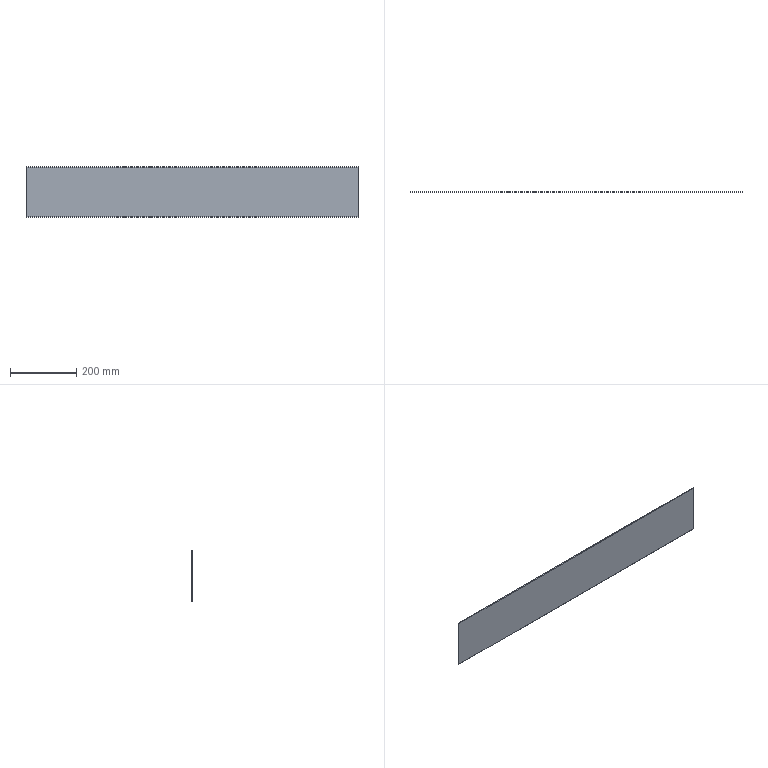Part | STEP file | 101000007619 | 1 solid | 8 faces | box 1000 x 2.5 x 152 mm | volume 378659 mm3 | plane 4 | cylinder 4 | commonest cylinder face diameters 2.5 x4
STEP:
#1=CARTESIAN_POINT('',(500.,0.,-74.75));
#2=VERTEX_POINT('',#1);
#3=CARTESIAN_POINT('',(500.,1.25,-76.));
#4=VERTEX_POINT('',#3);
#5=CARTESIAN_POINT('',(500.,0.,-74.75));
#6=CARTESIAN_POINT('',(500.,0.,-74.914));
#7=CARTESIAN_POINT('',(500.,0.027,-75.079));
#8=CARTESIAN_POINT('',(500.,0.08102,-75.237));
#9=CARTESIAN_POINT('',(500.,0.239,-75.53));
#10=CARTESIAN_POINT('',(500.,0.4826,-75.757));
#11=CARTESIAN_POINT('',(500.,0.6221,-75.85));
#12=CARTESIAN_POINT('',(500.,0.8334,-75.944));
#13=CARTESIAN_POINT('',(500.,1.058,-75.988));
#14=CARTESIAN_POINT('',(500.,1.122,-75.996));
#15=CARTESIAN_POINT('',(500.,1.186,-76.));
#16=CARTESIAN_POINT('',(500.,1.25,-76.));
#17=B_SPLINE_CURVE_WITH_KNOTS('',5,(#5,#6,#7,#8,#9,#10,#11,#12,#13,#14,#15,#16),.UNSPECIFIED.,.F.,.U.,(6,3,3,6),(0.,1.162,2.324,2.776),.UNSPECIFIED.);
#18=EDGE_CURVE('',#2,#4,#17,.T.);
#19=ORIENTED_EDGE('',*,*,#18,.T.);
#20=CARTESIAN_POINT('',(500.,2.5,-74.75));
#21=VERTEX_POINT('',#20);
#22=CARTESIAN_POINT('',(500.,1.25,-76.));
#23=CARTESIAN_POINT('',(500.,1.414,-76.));
#24=CARTESIAN_POINT('',(500.,1.579,-75.973));
#25=CARTESIAN_POINT('',(500.,1.737,-75.919));
#26=CARTESIAN_POINT('',(500.,2.03,-75.761));
#27=CARTESIAN_POINT('',(500.,2.257,-75.517));
#28=CARTESIAN_POINT('',(500.,2.35,-75.378));
#29=CARTESIAN_POINT('',(500.,2.444,-75.167));
#30=CARTESIAN_POINT('',(500.,2.488,-74.942));
#31=CARTESIAN_POINT('',(500.,2.496,-74.878));
#32=CARTESIAN_POINT('',(500.,2.5,-74.814));
#33=CARTESIAN_POINT('',(500.,2.5,-74.75));
#34=B_SPLINE_CURVE_WITH_KNOTS('',5,(#22,#23,#24,#25,#26,#27,#28,#29,#30,#31,#32,#33),.UNSPECIFIED.,.F.,.U.,(6,3,3,6),(0.,1.162,2.324,2.776),.UNSPECIFIED.);
#35=EDGE_CURVE('',#4,#21,#34,.T.);
#36=ORIENTED_EDGE('',*,*,#35,.T.);
#37=CARTESIAN_POINT('',(500.,2.5,74.75));
#38=VERTEX_POINT('',#37);
#39=CARTESIAN_POINT('',(500.,2.5,0.));
#40=DIRECTION('',(0.,0.,-1.));
#41=VECTOR('',#40,1.);
#42=LINE('',#39,#41);
#43=EDGE_CURVE('',#38,#21,#42,.T.);
#44=ORIENTED_EDGE('',*,*,#43,.F.);
#45=CARTESIAN_POINT('',(500.,1.25,76.));
#46=VERTEX_POINT('',#45);
#47=CARTESIAN_POINT('',(500.,2.5,74.75));
#48=CARTESIAN_POINT('',(500.,2.5,74.914));
#49=CARTESIAN_POINT('',(500.,2.473,75.079));
#50=CARTESIAN_POINT('',(500.,2.419,75.237));
#51=CARTESIAN_POINT('',(500.,2.261,75.53));
#52=CARTESIAN_POINT('',(500.,2.017,75.757));
#53=CARTESIAN_POINT('',(500.,1.878,75.85));
#54=CARTESIAN_POINT('',(500.,1.667,75.944));
#55=CARTESIAN_POINT('',(500.,1.442,75.988));
#56=CARTESIAN_POINT('',(500.,1.378,75.996));
#57=CARTESIAN_POINT('',(500.,1.314,76.));
#58=CARTESIAN_POINT('',(500.,1.25,76.));
#59=B_SPLINE_CURVE_WITH_KNOTS('',5,(#47,#48,#49,#50,#51,#52,#53,#54,#55,#56,#57,#58),.UNSPECIFIED.,.F.,.U.,(6,3,3,6),(0.,1.162,2.324,2.776),.UNSPECIFIED.);
#60=EDGE_CURVE('',#38,#46,#59,.T.);
#61=ORIENTED_EDGE('',*,*,#60,.T.);
#62=CARTESIAN_POINT('',(500.,0.,74.75));
#63=VERTEX_POINT('',#62);
#64=CARTESIAN_POINT('',(500.,1.25,76.));
#65=CARTESIAN_POINT('',(500.,1.086,76.));
#66=CARTESIAN_POINT('',(500.,0.9214,75.973));
#67=CARTESIAN_POINT('',(500.,0.763,75.919));
#68=CARTESIAN_POINT('',(500.,0.4698,75.761));
#69=CARTESIAN_POINT('',(500.,0.2426,75.517));
#70=CARTESIAN_POINT('',(500.,0.1502,75.378));
#71=CARTESIAN_POINT('',(500.,0.05608,75.167));
#72=CARTESIAN_POINT('',(500.,0.01235,74.942));
#73=CARTESIAN_POINT('',(500.,0.004093,74.878));
#74=CARTESIAN_POINT('',(500.,0.,74.814));
#75=CARTESIAN_POINT('',(500.,0.,74.75));
#76=B_SPLINE_CURVE_WITH_KNOTS('',5,(#64,#65,#66,#67,#68,#69,#70,#71,#72,#73,#74,#75),.UNSPECIFIED.,.F.,.U.,(6,3,3,6),(0.,1.162,2.324,2.776),.UNSPECIFIED.);
#77=EDGE_CURVE('',#46,#63,#76,.T.);
#78=ORIENTED_EDGE('',*,*,#77,.T.);
#79=CARTESIAN_POINT('',(500.,0.,0.));
#80=DIRECTION('',(0.,0.,-1.));
#81=VECTOR('',#80,1.);
#82=LINE('',#79,#81);
#83=EDGE_CURVE('',#63,#2,#82,.T.);
#84=ORIENTED_EDGE('',*,*,#83,.T.);
#85=EDGE_LOOP('',(#19,#36,#44,#61,#78,#84));
#86=FACE_OUTER_BOUND('',#85,.T.);
#87=CARTESIAN_POINT('',(500.,2.5,76.));
#88=DIRECTION('',(-1.,0.,0.));
#89=DIRECTION('',(0.,0.,1.));
#90=AXIS2_PLACEMENT_3D('',#87,#88,#89);
#91=PLANE('',#90);
#92=ADVANCED_FACE('',(#86),#91,.F.);
#93=CARTESIAN_POINT('',(-500.,1.25,-76.));
#94=VERTEX_POINT('',#93);
#95=CARTESIAN_POINT('',(-500.,1.25,-76.));
#96=DIRECTION('',(1.,0.,0.));
#97=VECTOR('',#96,1.);
#98=LINE('',#95,#97);
#99=EDGE_CURVE('',#4,#94,#98,.F.);
#100=ORIENTED_EDGE('',*,*,#99,.F.);
#101=ORIENTED_EDGE('',*,*,#18,.F.);
#102=CARTESIAN_POINT('',(-500.,0.,-74.75));
#103=VERTEX_POINT('',#102);
#104=CARTESIAN_POINT('',(-500.,0.,-74.75));
#105=DIRECTION('',(1.,0.,0.));
#106=VECTOR('',#105,1.);
#107=LINE('',#104,#106);
#108=EDGE_CURVE('',#103,#2,#107,.T.);
#109=ORIENTED_EDGE('',*,*,#108,.F.);
#110=CARTESIAN_POINT('',(-500.,1.25,-74.75));
#111=DIRECTION('',(1.,0.,0.));
#112=AXIS2_PLACEMENT_3D('',#110,#111,$);
#113=CIRCLE('',#112,1.25);
#114=EDGE_CURVE('',#94,#103,#113,.F.);
#115=ORIENTED_EDGE('',*,*,#114,.F.);
#116=EDGE_LOOP('',(#100,#101,#109,#115));
#117=FACE_OUTER_BOUND('',#116,.T.);
#118=CARTESIAN_POINT('',(-500.,1.25,-74.75));
#119=DIRECTION('',(1.,0.,0.));
#120=DIRECTION('',(0.,0.,1.));
#121=AXIS2_PLACEMENT_3D('',#118,#119,#120);
#122=CYLINDRICAL_SURFACE('',#121,1.25);
#123=ADVANCED_FACE('',(#117),#122,.T.);
#124=ORIENTED_EDGE('',*,*,#35,.F.);
#125=ORIENTED_EDGE('',*,*,#99,.T.);
#126=CARTESIAN_POINT('',(-500.,2.5,-74.75));
#127=VERTEX_POINT('',#126);
#128=CARTESIAN_POINT('',(-500.,1.25,-74.75));
#129=DIRECTION('',(-1.,0.,0.));
#130=AXIS2_PLACEMENT_3D('',#128,#129,$);
#131=CIRCLE('',#130,1.25);
#132=EDGE_CURVE('',#127,#94,#131,.T.);
#133=ORIENTED_EDGE('',*,*,#132,.F.);
#134=CARTESIAN_POINT('',(0.,2.5,-74.75));
#135=DIRECTION('',(-1.,0.,0.));
#136=VECTOR('',#135,1.);
#137=LINE('',#134,#136);
#138=EDGE_CURVE('',#21,#127,#137,.T.);
#139=ORIENTED_EDGE('',*,*,#138,.F.);
#140=EDGE_LOOP('',(#124,#125,#133,#139));
#141=FACE_OUTER_BOUND('',#140,.T.);
#142=CARTESIAN_POINT('',(0.,1.25,-74.75));
#143=DIRECTION('',(-1.,0.,0.));
#144=DIRECTION('',(0.,0.,1.));
#145=AXIS2_PLACEMENT_3D('',#142,#143,#144);
#146=CYLINDRICAL_SURFACE('',#145,1.25);
#147=ADVANCED_FACE('',(#141),#146,.T.);
#148=ORIENTED_EDGE('',*,*,#43,.T.);
#149=ORIENTED_EDGE('',*,*,#138,.T.);
#150=CARTESIAN_POINT('',(-500.,2.5,74.75));
#151=VERTEX_POINT('',#150);
#152=CARTESIAN_POINT('',(-500.,2.5,0.));
#153=DIRECTION('',(0.,0.,1.));
#154=VECTOR('',#153,1.);
#155=LINE('',#152,#154);
#156=EDGE_CURVE('',#127,#151,#155,.T.);
#157=ORIENTED_EDGE('',*,*,#156,.T.);
#158=CARTESIAN_POINT('',(0.,2.5,74.75));
#159=DIRECTION('',(1.,0.,0.));
#160=VECTOR('',#159,1.);
#161=LINE('',#158,#160);
#162=EDGE_CURVE('',#151,#38,#161,.T.);
#163=ORIENTED_EDGE('',*,*,#162,.T.);
#164=EDGE_LOOP('',(#148,#149,#157,#163));
#165=FACE_OUTER_BOUND('',#164,.T.);
#166=CARTESIAN_POINT('',(0.,2.5,0.));
#167=DIRECTION('',(0.,-1.,0.));
#168=DIRECTION('',(0.,0.,-1.));
#169=AXIS2_PLACEMENT_3D('',#166,#167,#168);
#170=PLANE('',#169);
#171=ADVANCED_FACE('',(#165),#170,.F.);
#172=ORIENTED_EDGE('',*,*,#162,.F.);
#173=CARTESIAN_POINT('',(-500.,1.25,76.));
#174=VERTEX_POINT('',#173);
#175=CARTESIAN_POINT('',(-500.,1.25,74.75));
#176=DIRECTION('',(1.,0.,0.));
#177=AXIS2_PLACEMENT_3D('',#175,#176,$);
#178=CIRCLE('',#177,1.25);
#179=EDGE_CURVE('',#174,#151,#178,.F.);
#180=ORIENTED_EDGE('',*,*,#179,.F.);
#181=CARTESIAN_POINT('',(0.,1.25,76.));
#182=DIRECTION('',(1.,0.,0.));
#183=VECTOR('',#182,1.);
#184=LINE('',#181,#183);
#185=EDGE_CURVE('',#46,#174,#184,.F.);
#186=ORIENTED_EDGE('',*,*,#185,.F.);
#187=ORIENTED_EDGE('',*,*,#60,.F.);
#188=EDGE_LOOP('',(#172,#180,#186,#187));
#189=FACE_OUTER_BOUND('',#188,.T.);
#190=CARTESIAN_POINT('',(0.,1.25,74.75));
#191=DIRECTION('',(1.,0.,0.));
#192=DIRECTION('',(0.,0.,-1.));
#193=AXIS2_PLACEMENT_3D('',#190,#191,#192);
#194=CYLINDRICAL_SURFACE('',#193,1.25);
#195=ADVANCED_FACE('',(#189),#194,.T.);
#196=CARTESIAN_POINT('',(-500.,0.,74.75));
#197=VERTEX_POINT('',#196);
#198=CARTESIAN_POINT('',(-500.,1.25,74.75));
#199=DIRECTION('',(-1.,0.,0.));
#200=AXIS2_PLACEMENT_3D('',#198,#199,$);
#201=CIRCLE('',#200,1.25);
#202=EDGE_CURVE('',#197,#174,#201,.T.);
#203=ORIENTED_EDGE('',*,*,#202,.F.);
#204=CARTESIAN_POINT('',(-500.,0.,74.75));
#205=DIRECTION('',(-1.,0.,0.));
#206=VECTOR('',#205,1.);
#207=LINE('',#204,#206);
#208=EDGE_CURVE('',#63,#197,#207,.T.);
#209=ORIENTED_EDGE('',*,*,#208,.F.);
#210=ORIENTED_EDGE('',*,*,#77,.F.);
#211=ORIENTED_EDGE('',*,*,#185,.T.);
#212=EDGE_LOOP('',(#203,#209,#210,#211));
#213=FACE_OUTER_BOUND('',#212,.T.);
#214=CARTESIAN_POINT('',(-500.,1.25,74.75));
#215=DIRECTION('',(-1.,0.,0.));
#216=DIRECTION('',(0.,0.,-1.));
#217=AXIS2_PLACEMENT_3D('',#214,#215,#216);
#218=CYLINDRICAL_SURFACE('',#217,1.25);
#219=ADVANCED_FACE('',(#213),#218,.T.);
#220=CARTESIAN_POINT('',(-500.,0.,0.));
#221=DIRECTION('',(0.,0.,1.));
#222=VECTOR('',#221,1.);
#223=LINE('',#220,#222);
#224=EDGE_CURVE('',#103,#197,#223,.T.);
#225=ORIENTED_EDGE('',*,*,#224,.F.);
#226=ORIENTED_EDGE('',*,*,#108,.T.);
#227=ORIENTED_EDGE('',*,*,#83,.F.);
#228=ORIENTED_EDGE('',*,*,#208,.T.);
#229=EDGE_LOOP('',(#225,#226,#227,#228));
#230=FACE_OUTER_BOUND('',#229,.T.);
#231=CARTESIAN_POINT('',(0.,0.,0.));
#232=DIRECTION('',(0.,-1.,0.));
#233=DIRECTION('',(0.,0.,-1.));
#234=AXIS2_PLACEMENT_3D('',#231,#232,#233);
#235=PLANE('',#234);
#236=ADVANCED_FACE('',(#230),#235,.T.);
#237=ORIENTED_EDGE('',*,*,#156,.F.);
#238=ORIENTED_EDGE('',*,*,#132,.T.);
#239=ORIENTED_EDGE('',*,*,#114,.T.);
#240=ORIENTED_EDGE('',*,*,#224,.T.);
#241=ORIENTED_EDGE('',*,*,#202,.T.);
#242=ORIENTED_EDGE('',*,*,#179,.T.);
#243=EDGE_LOOP('',(#237,#238,#239,#240,#241,#242));
#244=FACE_OUTER_BOUND('',#243,.T.);
#245=CARTESIAN_POINT('',(-500.,2.5,76.));
#246=DIRECTION('',(1.,0.,0.));
#247=DIRECTION('',(0.,0.,-1.));
#248=AXIS2_PLACEMENT_3D('',#245,#246,#247);
#249=PLANE('',#248);
#250=ADVANCED_FACE('',(#244),#249,.F.);
#251=CLOSED_SHELL('',(#92,#123,#147,#171,#195,#219,#236,#250));
#252=MANIFOLD_SOLID_BREP('',#251);
#253=(LENGTH_UNIT()NAMED_UNIT(*)SI_UNIT(.MILLI.,.METRE.));
#254=UNCERTAINTY_MEASURE_WITH_UNIT(LENGTH_MEASURE(0.005),#253,'','');
#255=(NAMED_UNIT(*)PLANE_ANGLE_UNIT()SI_UNIT($,.RADIAN.));
#256=(NAMED_UNIT(*)SI_UNIT($,.STERADIAN.)SOLID_ANGLE_UNIT());
#257=(GEOMETRIC_REPRESENTATION_CONTEXT(3)GLOBAL_UNCERTAINTY_ASSIGNED_CONTEXT((#254))GLOBAL_UNIT_ASSIGNED_CONTEXT((#253,#255,#256))REPRESENTATION_CONTEXT('',''));
#258=ADVANCED_BREP_SHAPE_REPRESENTATION('',(#252),#257);